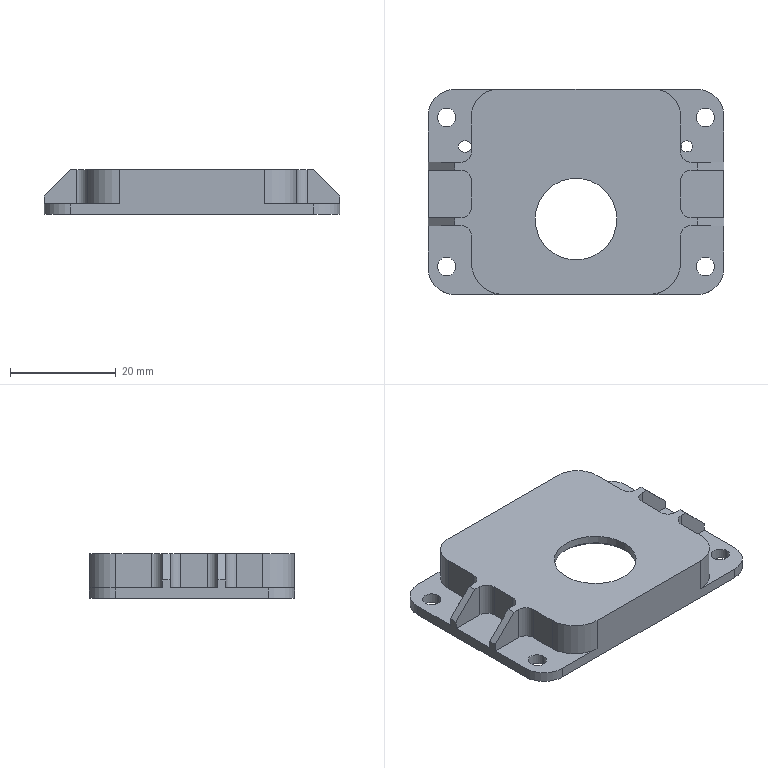NC program | NX | posted with a generic post | part box 56 x 38.85 x 8.5 mm
Lines 1 to 290 of 3190:
N10 G17 G21 G94 G90
(FLOOR_WALL_COPY_COPY , TOOL : D80)
N12 T19 M6
N14 G54
N16 G17 G0 G90 X-73. Y0. S6500 M3
N18 G43 Z30. H19
N20 Z5.625
N22 G94 G1 Z2.625 F1500.
N24 X-68.
N26 X68.
N28 X73.
N30 Z5.625
N32 G0 Z30.
N34 X-73.
N36 Z4.75
N38 G1 Z1.75
N40 X-68.
N42 X68.
N44 X73.
N46 Z4.75
N48 G0 Z30.
N50 X-73.
N52 Z3.875
N54 G1 Z0.875
N56 X-68.
N58 X68.
N60 X73.
N62 Z3.875
N64 G0 Z30.
N66 X-73.
N68 Z3.
N70 G1 Z0.
N72 X-68.
N74 X68.
N76 X73.
N78 Z3.
N80 G0 Z30.
N82 M5
(DRILLING_COPY_1_COPY , TOOL : D6A45)
N84 T01 M6
N86 G54
N88 G17 G0 G90 X24.5 Y14.125 S5000 M3
N90 G43 Z30. H1
N92 G94 G81 G98 Z-1.55 F350. R3.
N94 Y-14.125
N96 X-24.5
N98 X-21. Y8.625
N100 X-24.5 Y14.125
N102 G80
N104 G0 X-24.5 Y14.125 Z30.
N106 M5
(DRILLING_COPY_1_COPY_1_1_COPY_1 , TOOL : 2.1ZT)
N108 T02 M6
N110 G54
N112 G17 G0 G90 X-21. Y8.625 S2000 M3
N114 G43 Z30. H2
N116 G94 G83 G98 Z-4.131 F120. Q2. R3.
N118 G80
N120 G0 X-21. Y8.625 Z30.
N122 M5
(DRILLING_COPY_1_COPY_1_1_COPY_1_COPY , TOOL : 3.5ZT)
N124 T07 M6
N126 G54
N128 G17 G0 G90 X-24.5 Y-14.125 S2000 M3
N130 G43 Z30. H7
N132 G94 G83 G98 Z-4.552 F120. Q2. R3.
N134 Y14.125
N136 X24.5
N138 Y-14.125
N140 G80
N142 G0 X24.5 Y-14.125 Z30.
N144 M5
(CAVITY_MILL_COPY_1 , TOOL : D10)
N146 T15 M6
N148 G54
N150 G17 G0 G90 X0.866 Y-0.275 S9500 M3
N152 G43 Z30. H15
N154 Z0.05
N156 G94 G1 Z-0.95 F1000.
N158 G3 X0. Y0.225 R1.
N160 G1 X-0.6 F2500.
N162 Y-0.225
N164 X0.6
N166 Y0.225
N168 X0.
N170 Y6.225
N172 X-6.6
N174 Y-6.225
N176 X6.6
N178 Y6.225
N180 X0.
N182 Y12.225
N184 X-12.6
N186 Y-12.225
N188 X12.6
N190 Y12.225
N192 X0.
N194 G3 X-0.866 Y11.725 R1.
N196 G1 Z0.05
N198 G0 X0.866 Y-0.275 Z-0.9
N200 G1 Z-1.9 F1000.
N202 G3 X0. Y0.225 R1.
N204 G1 X-0.6 F2500.
N206 Y-0.225
N208 X0.6
N210 Y0.225
N212 X0.
N214 Y6.225
N216 X-6.6
N218 Y-6.225
N220 X6.6
N222 Y6.225
N224 X0.
N226 Y12.225
N228 X-12.6
N230 Y-12.225
N232 X12.6
N234 Y12.225
N236 X0.
N238 G3 X-0.866 Y11.725 R1.
N240 G1 Z-0.9
N242 G0 X0.866 Y-0.275 Z-1.65
N244 G1 Z-2.65 F1000.
N246 G3 X0. Y0.225 R1.
N248 G1 X-0.6 F2500.
N250 Y-0.225
N252 X0.6
N254 Y0.225
N256 X0.
N258 Y6.225
N260 X-6.6
N262 Y-6.225
N264 X6.6
N266 Y6.225
N268 X0.
N270 Y12.225
N272 X-12.6
N274 Y-12.225
N276 X12.6
N278 Y12.225
N280 X0.
N282 G3 X-0.866 Y11.725 R1.
N284 G1 Z-1.65
N286 G0 X0.866 Y-0.275 Z-2.4
N288 G1 Z-3.4 F1000.
N290 G3 X0. Y0.225 R1.
N292 G1 X-0.6 F2500.
N294 Y-0.225
N296 X0.6
N298 Y0.225
N300 X0.
N302 Y6.225
N304 X-6.6
N306 Y-6.225
N308 X6.6
N310 Y6.225
N312 X0.
N314 Y12.225
N316 X-12.6
N318 Y-12.225
N320 X12.6
N322 Y12.225
N324 X0.
N326 G3 X-0.866 Y11.725 R1.
N328 G1 Z-2.4
N330 G0 X0.4 Y-3.784 Z-3.4
N332 G1 Z-4.4 F1000.
N334 G3 X-0.1 Y-4.65 R1.
N336 G1 Y-5.898 F2500.
N338 X-0.101 Y-6.027
N340 X0. Y-6.13
N342 X0.101 Y-6.027
N344 X0.1 Y-5.898
N346 Y-4.398
N348 G2 X0.157 Y-3.275 R11.1
N350 G1 X-0.157
N352 G2 X-0.1 Y-4.398 R11.1
N354 G1 Y-4.65
N356 X-6.1
N358 Y-5.898
N360 G2 X-7.019 Y-8.819 R5.1
N362 G1 X-6.923 Y-8.84
N364 G2 X-3.157 Y-12.225 R5.1
N366 G1 X3.157
N368 G2 X6.923 Y-8.84 R5.1
N370 G1 X7.019 Y-8.819
N372 G2 X6.1 Y-5.898 R5.1
N374 G1 Y-4.398
N376 G2 X7.17 Y-1.273 R5.1
N378 X6.1 Y1.852 R5.1
N380 G1 Y3.092
N382 G2 X4.375 Y4.238 R5.1
N384 X0.75 Y2.725 R5.1
N386 G1 X-0.75
N388 G2 X-4.375 Y4.238 R5.1
N390 X-6.1 Y3.092 R5.1
N392 G1 Y1.852
N394 G2 X-7.17 Y-1.273 R5.1
N396 X-6.1 Y-4.398 R5.1
N398 G1 Y-4.65
N400 G3 X-5.6 Y-5.516 R1.
N402 G1 Z-3.4
N404 G0 X-0.4 Z-4.4
N406 G1 Z-5.4 F1000.
N408 G3 X0.1 Y-4.65 R1.
N410 G1 Y-4.398 F2500.
N412 G2 X0.157 Y-3.275 R11.1
N414 G1 X-0.157
N416 G2 X-0.1 Y-4.398 R11.1
N418 G1 Y-5.898
N420 X-0.101 Y-6.027
N422 X0. Y-6.13
N424 X0.101 Y-6.027
N426 X0.1 Y-5.898
N428 Y-4.65
N430 X6.1
N432 Y-4.398
N434 G2 X7.17 Y-1.273 R5.1
N436 X6.1 Y1.852 R5.1
N438 G1 Y3.092
N440 G2 X4.375 Y4.238 R5.1
N442 X0.75 Y2.725 R5.1
N444 G1 X-0.75
N446 G2 X-4.375 Y4.238 R5.1
N448 X-6.1 Y3.092 R5.1
N450 G1 Y1.852
N452 G2 X-7.17 Y-1.273 R5.1
N454 X-6.1 Y-4.398 R5.1
N456 G1 Y-5.898
N458 G2 X-7.019 Y-8.819 R5.1
N460 G1 X-6.923 Y-8.84
N462 G2 X-3.157 Y-12.225 R5.1
N464 G1 X3.157
N466 G2 X6.923 Y-8.84 R5.1
N468 G1 X7.019 Y-8.819
N470 G2 X6.1 Y-5.898 R5.1
N472 G1 Y-4.65
N474 G3 X5.6 Y-3.784 R1.
N476 G1 Z-4.4
N478 G0 X0.4 Z-5.4
N480 G1 Z-6.4 F1000.
N482 G3 X-0.1 Y-4.65 R1.
N484 G1 Y-5.898 F2500.
N486 X-0.101 Y-6.027
N488 X0. Y-6.13
N490 X0.101 Y-6.027
N492 X0.1 Y-5.898
N494 Y-4.398
N496 G2 X0.157 Y-3.275 R11.1
N498 G1 X-0.157
N500 G2 X-0.1 Y-4.398 R11.1
N502 G1 Y-4.65
N504 X-6.1
N506 Y-5.898
N508 G2 X-7.019 Y-8.819 R5.1
N510 G1 X-6.923 Y-8.84
N512 G2 X-3.157 Y-12.225 R5.1
N514 G1 X3.157
N516 G2 X6.923 Y-8.84 R5.1
N518 G1 X7.019 Y-8.819
N520 G2 X6.1 Y-5.898 R5.1
N522 G1 Y-4.398
N524 G2 X7.17 Y-1.273 R5.1
N526 X6.1 Y1.852 R5.1
N528 G1 Y3.092
N530 G2 X4.375 Y4.238 R5.1
N532 X0.75 Y2.725 R5.1
N534 G1 X-0.75
N536 G2 X-4.375 Y4.238 R5.1
N538 X-6.1 Y3.092 R5.1
N540 G1 Y1.852
N542 G2 X-7.17 Y-1.273 R5.1
N544 X-6.1 Y-4.398 R5.1
N546 G1 Y-4.65
N548 G3 X-5.6 Y-5.516 R1.
N550 G1 Z-5.4
N552 G0 Z30.
N554 M5